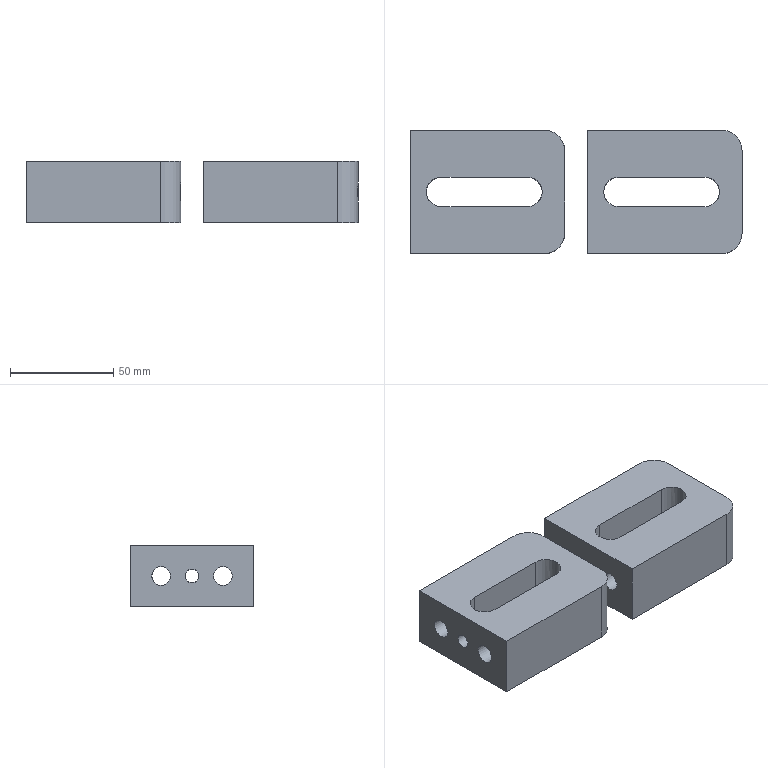CAM job | NX | 3-axis milling, drilling | part box 161 x 60 x 30 mm | stock box 166 x 65 x 35 mm
Tools:
number,name,description,diameter,corner_radius,flute_length,length,flutes
9,D10,平底铣刀-粗,10.0,0.0,35.0,75.0,2
10,D10-J,平底铣刀-精,10.0,0.0,35.0,75.0,2
1,D80R0.8飞刀,圆鼻刀-粗,80.0,0.8,50.0,75.0,2
1,D80R0.8飞刀-J,圆鼻刀-精,80.0,0.8,50.0,75.0,2
2,D6倒角刀,倒角刀,6.0,0.0,3.0,25.0,2
17,ZT9.5,钻头,9.5,0.0,35.0,50.0,2
Operations:
program,operation,operation_type,tool,method,geometry_group,spindle_rpm,surface_speed,feed_per_tooth,feed_cut,feed_plunge,cut_length_mm,path_length_mm,cut_time_min,machine_time_min
B,底壁铣飞面一刀开粗_COPY,VolumeBased25DMillingOperation,D80R0.8飞刀,分层开粗-切深K-步距G,W-B,2800.0,703.696,0.5357,3000.0,100.0,2422.746,4742.966,0.8076,1.04
B,底壁铣飞面一刀精光_COPY,VolumeBased25DMillingOperation,D80R0.8飞刀-J,侧刃精光-切深K-步距G,W-B,4000.0,1005.28,0.125,1000.0,100.0,268.998,304.998,0.269,0.2726
B,C0.3平面去毛刺6X45L__COPY,SurfaceContour,D6倒角刀,爬面_倒角-切深0-步距G,W-B,8000.0,150.796,0.0938,1500.0,90.0,795.459,1078.872,0.5309,0.5592
A,顶面,FaceMilling,D80R0.8飞刀,侧刃精光-切深K-步距G,W-A,4000.0,1005.31,0.125,1000.0,100.0,255.0,291.0,0.255,0.2586
A,外形粗_2,VolumeBased25DMillingOperation,D10,METHOD,W-A,8000.0,251.327,0.3125,5000.0,80.0,23479.897,23703.997,4.696,4.718
A,打点,Operation,D6倒角刀,METHOD,W-A,3000.0,56.0,0.0333,200.0,0.0,10.2,191.435,0.051,0.0691
A,预钻孔8,Operation,ZT9.5,METHOD,W-A,1200.0,35.814,0.1042,250.0,0.0,156.0,483.035,0.624,0.6567
A,通腰槽粗_1,VolumeBased25DMillingOperation,D10,METHOD,W-A,8000.0,251.327,0.1562,2500.0,100.0,12170.52,12393.42,4.868,4.891
A,腰槽精_1,VolumeBased25DMillingOperation,D10-J,METHOD,W-A,6000.0,113.0,0.0667,600.0,100.0,1193.076,1596.643,1.988,2.029
A,仅选体,SurfaceContour,D6倒角刀,METHOD,W-A,8000.0,150.796,0.1875,3000.0,100.0,816.64,1074.295,0.2722,0.298
A,外形半精_2,VolumeBased25DMillingOperation,D10-J,METHOD,W-A,8000.0,251.327,0.0625,1000.0,100.0,1191.431,1736.237,1.191,1.246